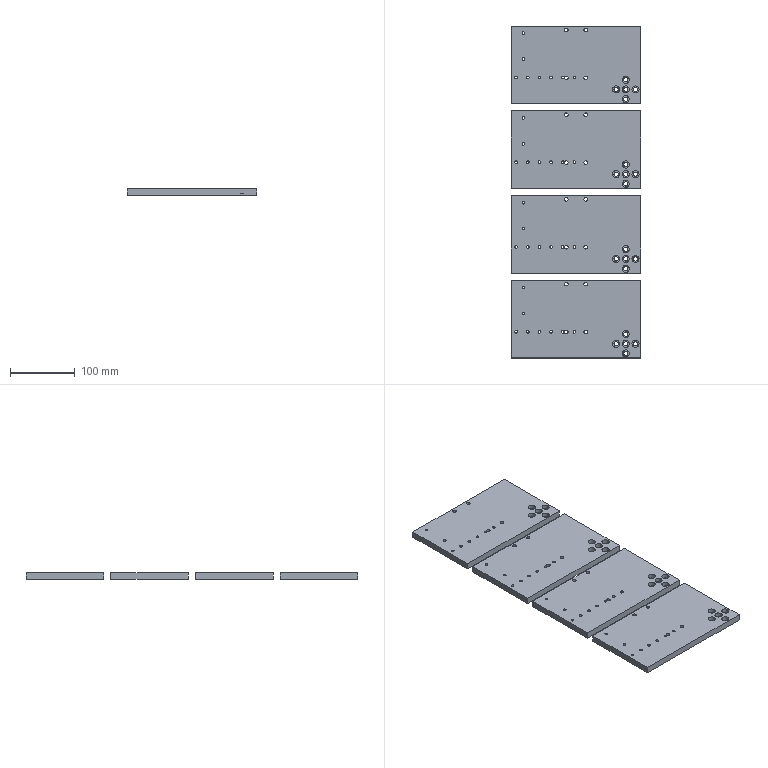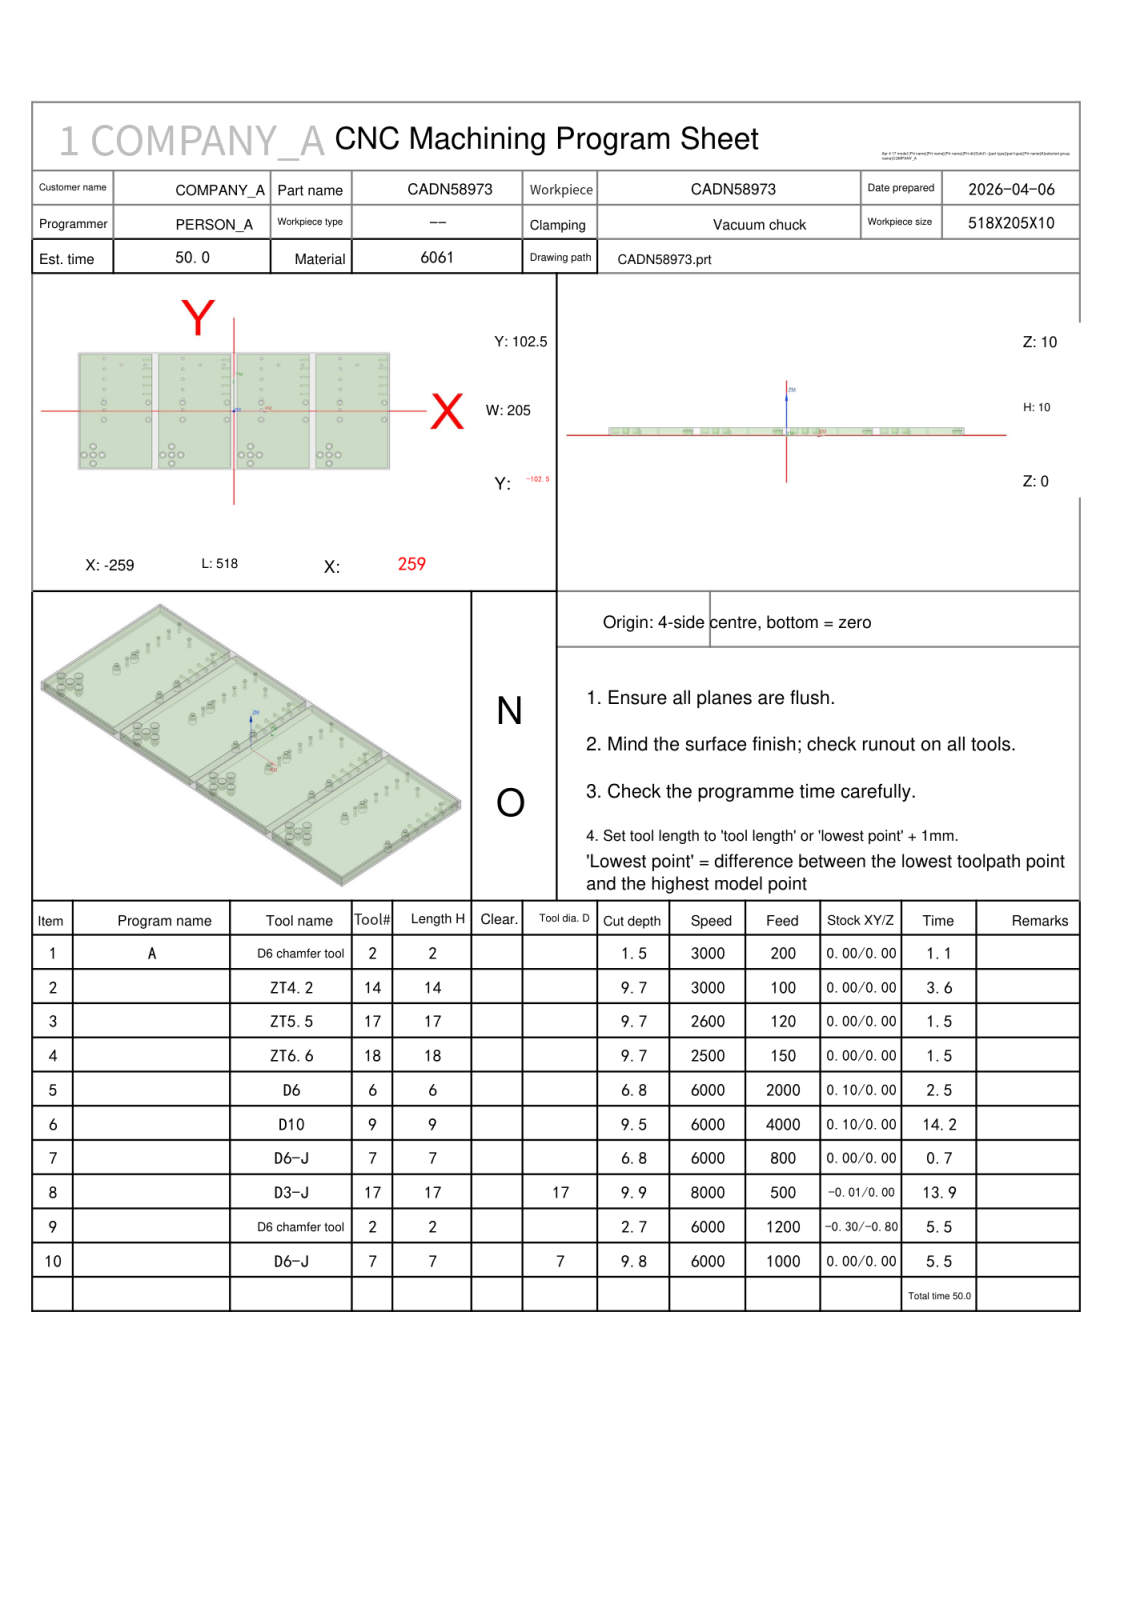NC program | NX | posted by the shop | part box 200 x 513 x 10 mm
Lines 1 to 1767 of 10035, first 1367 of 1765 lines:
%
O0001
(Machine time: 51.42 MIN)
(===Total Tool:7===)
(T2=D6 chamfer tool   D=6.   R=0.   D-  H02 Z=7.33  )
(T14=ZT4.2  D=4.2  DR_a=118 D-  H14 Z=0.3   )
(T17=ZT5.5  D=5.5  DR_a=118 D-  H17 Z=0.15  )
(T18=ZT6.6  D=6.6  DR_a=118 D-  H18 Z=0.3   )
(T6=D6      D=6.   R=0.   D-  H06 Z=3.2   )
(T9=D10     D=10.  R=0.   D-  H09 Z=0.5   )
(T7=D6-J    D=6.   R=0.   D-  H07 Z=0.2   )
G80 G90 G17 G49 G40
G91 G28 Z0
M01
N1 T02 M06
(D6 chamfer tool  D=6. R=0. H=02 ce=0.00 di=0.00)
G00 G90 G54 X-219.5 Y-77. M03 S3000
G43 H02 Z30.
M08
G98 G81 X-219.5 Y-77. Z8.5 R11. F200.
X-234.5
Y-92.
X-249.5 Y-77.
X-234.5 Y-62.
X-216.5 Y-15.
X-216. Y2.515
X-216.5 Y15.
X-216. Y20.515
Y38.515
Y56.515
Y74.515
Y92.515
X-187.5 Y81.264
X-147.5
X-85. Y92.515
X-16.5 Y81.264
X-56.5
X-85. Y74.515
Y56.515
Y38.515
Y20.515
X-85.5 Y15.
X-142.5
Y-15.
X-118.5 Y-77.
X-103.5 Y-92.
X-88.5 Y-77.
X-103.5
Y-62.
X-85.5 Y-15.
X-85. Y2.515
X-11.5 Y15.
Y-15.
X12.5 Y-77.
X27.5
Y-92.
X42.5 Y-77.
X27.5 Y-62.
X45.5 Y-15.
X46. Y2.515
X45.5 Y15.
X46. Y20.515
Y38.515
Y56.515
Y74.515
Y92.515
X74.5 Y81.264
X114.5
X119.5 Y15.
Y-15.
X158.5 Y-62.
Y-77.
X143.5
X158.5 Y-92.
X173.5 Y-77.
X176.5 Y-15.
X177. Y2.515
X176.5 Y15.
X177. Y20.515
Y38.515
Y56.515
Y74.515
Y92.515
X205.5 Y81.264
X245.5
X250.5 Y15.
Y-15.
G80
G00 Z30.
G91 G28 Z0.0
M05
M09
G91 G28 Z0.0
M01
N2 T14 M06
(ZT4.2 D=4.2 DR_a=118 H=14)
G00 G90 G54 X-216. Y2.515 M03 S3000
G43 H14 Z30.
M08
G98 G83 X-216. Y2.515 Z.3 R11. F100. Q1.5
Y20.515
Y38.515
Y56.515
Y74.515
Y92.515
X-187.5 Y81.264
X-147.5
X-85. Y2.515
Y20.515
Y38.515
Y56.515
Y74.515
Y92.515
X-56.5 Y81.264
X-16.5
X46. Y2.515
Y20.515
Y38.515
Y56.515
Y74.515
Y92.515
X74.5 Y81.264
X114.5
X177. Y92.515
X245.5 Y81.264
X205.5
X177. Y74.515
Y56.515
Y38.515
Y20.515
Y2.515
G80
G00 Z30.
G91 G28 Z0.0
M05
M09
G91 G28 Z0.0
M01
N3 T17 M06
(ZT5.5 D=5.5 DR_a=118 H=17)
G00 G90 G54 X250.5 Y15. M03 S2600
G43 H17 Z30.
M08
G98 G83 X250.5 Y15. Z.3 R11. F120. Q1.5
Y-15.
X176.5
Y15.
X119.5
Y-15.
X45.5
Y15.
X-11.5
Y-15.
X-85.5
Y15.
X-142.5
Y-15.
X-216.5
Y15.
G80
G00 Z30.
G91 G28 Z0.0
M05
M09
G91 G28 Z0.0
M01
N4 T18 M06
(ZT6.6 D=6.6 DR_a=118 H=18)
G00 G90 G54 X-234.5 Y-92. M03 S2500
G43 H18 Z30.
M08
G98 G83 X-234.5 Y-92. Z.3 R11. F150. Q3.
X-249.5 Y-77.
X-234.5
Y-62.
X-219.5 Y-77.
X-118.5
X-103.5 Y-62.
Y-77.
Y-92.
X-88.5 Y-77.
X12.5
X27.5 Y-92.
Y-77.
Y-62.
X42.5 Y-77.
X143.5
X158.5 Y-92.
Y-77.
Y-62.
X173.5 Y-77.
G80
G00 Z30.
G91 G28 Z0.0
M05
M09
G91 G28 Z0.0
M01
N5 T06 M06
(D6  D=6. R=0. H=06 ce=0.10 di=0.00)
G00 G90 G54 X42.5 Y-77. M03 S6000
G43 H06 Z30.
M08
Z10.3
G03 X41.3 Y-78.2 I0.0 J-1.2 F2000.
X42.5 Y-79.4 I1.2 J0.0
X42.5 Y-79.4 Z9.8 I0.0 J2.4
X42.5 Y-79.4 Z9.3 I0.0 J2.4
X42.5 Y-79.4 Z8.8 I0.0 J2.4
X42.5 Y-79.4 Z8.3 I0.0 J2.4
X42.5 Y-79.4 Z7.8 I0.0 J2.4
X42.5 Y-79.4 Z7.3 I0.0 J2.4
X42.5 Y-79.4 Z6.8 I0.0 J2.4
X42.5 Y-79.4 Z6.3 I0.0 J2.4
X42.5 Y-79.4 Z5.8 I0.0 J2.4
X42.5 Y-79.4 Z5.3 I0.0 J2.4
X42.5 Y-79.4 Z4.8 I0.0 J2.4
X42.5 Y-79.4 Z4.3 I0.0 J2.4
X42.5 Y-79.4 Z3.8 I0.0 J2.4
X42.5 Y-79.4 Z3.3 I0.0 J2.4
X44.783 Y-77.742 Z3.2 I0.0 J2.4
X44.9 Y-77. I-2.283 J.742
X42.5 Y-74.6 I-2.4 J0.0
X40.1 Y-77. I0.0 J-2.4
X42.5 Y-79.4 I2.4 J0.0
X44.783 Y-77.742 I0.0 J2.4
X44.841 Y-77.371 I-1.141 J.371
X43.641 Y-76.171 I-1.2 J0.0
X42.5 Y-77. I0.0 J-1.2
G00 Z30.
X143.5
Z10.3
G03 X142.3 Y-78.2 I0.0 J-1.2
X143.5 Y-79.4 I1.2 J0.0
X143.5 Y-79.4 Z9.8 I0.0 J2.4
X143.5 Y-79.4 Z9.3 I0.0 J2.4
X143.5 Y-79.4 Z8.8 I0.0 J2.4
X143.5 Y-79.4 Z8.3 I0.0 J2.4
X143.5 Y-79.4 Z7.8 I0.0 J2.4
X143.5 Y-79.4 Z7.3 I0.0 J2.4
X143.5 Y-79.4 Z6.8 I0.0 J2.4
X143.5 Y-79.4 Z6.3 I0.0 J2.4
X143.5 Y-79.4 Z5.8 I0.0 J2.4
X143.5 Y-79.4 Z5.3 I0.0 J2.4
X143.5 Y-79.4 Z4.8 I0.0 J2.4
X143.5 Y-79.4 Z4.3 I0.0 J2.4
X143.5 Y-79.4 Z3.8 I0.0 J2.4
X143.5 Y-79.4 Z3.3 I0.0 J2.4
X145.783 Y-77.742 Z3.2 I0.0 J2.4
X145.9 Y-77. I-2.283 J.742
X143.5 Y-74.6 I-2.4 J0.0
X141.1 Y-77. I0.0 J-2.4
X143.5 Y-79.4 I2.4 J0.0
X145.783 Y-77.742 I0.0 J2.4
X145.841 Y-77.371 I-1.141 J.371
X144.641 Y-76.171 I-1.2 J0.0
X143.5 Y-77. I0.0 J-1.2
G00 Z30.
X158.5 Y-92.
Z10.3
G03 X157.3 Y-93.2 I0.0 J-1.2
X158.5 Y-94.4 I1.2 J0.0
X158.5 Y-94.4 Z9.8 I0.0 J2.4
X158.5 Y-94.4 Z9.3 I0.0 J2.4
X158.5 Y-94.4 Z8.8 I0.0 J2.4
X158.5 Y-94.4 Z8.3 I0.0 J2.4
X158.5 Y-94.4 Z7.8 I0.0 J2.4
X158.5 Y-94.4 Z7.3 I0.0 J2.4
X158.5 Y-94.4 Z6.8 I0.0 J2.4
X158.5 Y-94.4 Z6.3 I0.0 J2.4
X158.5 Y-94.4 Z5.8 I0.0 J2.4
X158.5 Y-94.4 Z5.3 I0.0 J2.4
X158.5 Y-94.4 Z4.8 I0.0 J2.4
X158.5 Y-94.4 Z4.3 I0.0 J2.4
X158.5 Y-94.4 Z3.8 I0.0 J2.4
X158.5 Y-94.4 Z3.3 I0.0 J2.4
X160.783 Y-92.742 Z3.2 I0.0 J2.4
X160.9 Y-92. I-2.283 J.742
X158.5 Y-89.6 I-2.4 J0.0
X156.1 Y-92. I0.0 J-2.4
X158.5 Y-94.4 I2.4 J0.0
X160.783 Y-92.742 I0.0 J2.4
X160.841 Y-92.371 I-1.141 J.371
X159.641 Y-91.171 I-1.2 J0.0
X158.5 Y-92. I0.0 J-1.2
G00 Z30.
Y-77.
Z10.3
G03 X157.3 Y-78.2 I0.0 J-1.2
X158.5 Y-79.4 I1.2 J0.0
X158.5 Y-79.4 Z9.8 I0.0 J2.4
X158.5 Y-79.4 Z9.3 I0.0 J2.4
X158.5 Y-79.4 Z8.8 I0.0 J2.4
X158.5 Y-79.4 Z8.3 I0.0 J2.4
X158.5 Y-79.4 Z7.8 I0.0 J2.4
X158.5 Y-79.4 Z7.3 I0.0 J2.4
X158.5 Y-79.4 Z6.8 I0.0 J2.4
X158.5 Y-79.4 Z6.3 I0.0 J2.4
X158.5 Y-79.4 Z5.8 I0.0 J2.4
X158.5 Y-79.4 Z5.3 I0.0 J2.4
X158.5 Y-79.4 Z4.8 I0.0 J2.4
X158.5 Y-79.4 Z4.3 I0.0 J2.4
X158.5 Y-79.4 Z3.8 I0.0 J2.4
X158.5 Y-79.4 Z3.3 I0.0 J2.4
X160.783 Y-77.742 Z3.2 I0.0 J2.4
X160.9 Y-77. I-2.283 J.742
X158.5 Y-74.6 I-2.4 J0.0
X156.1 Y-77. I0.0 J-2.4
X158.5 Y-79.4 I2.4 J0.0
X160.783 Y-77.742 I0.0 J2.4
X160.841 Y-77.371 I-1.141 J.371
X159.641 Y-76.171 I-1.2 J0.0
X158.5 Y-77. I0.0 J-1.2
G00 Z30.
X173.5
Z10.3
G03 X172.3 Y-78.2 I0.0 J-1.2
X173.5 Y-79.4 I1.2 J0.0
X173.5 Y-79.4 Z9.8 I0.0 J2.4
X173.5 Y-79.4 Z9.3 I0.0 J2.4
X173.5 Y-79.4 Z8.8 I0.0 J2.4
X173.5 Y-79.4 Z8.3 I0.0 J2.4
X173.5 Y-79.4 Z7.8 I0.0 J2.4
X173.5 Y-79.4 Z7.3 I0.0 J2.4
X173.5 Y-79.4 Z6.8 I0.0 J2.4
X173.5 Y-79.4 Z6.3 I0.0 J2.4
X173.5 Y-79.4 Z5.8 I0.0 J2.4
X173.5 Y-79.4 Z5.3 I0.0 J2.4
X173.5 Y-79.4 Z4.8 I0.0 J2.4
X173.5 Y-79.4 Z4.3 I0.0 J2.4
X173.5 Y-79.4 Z3.8 I0.0 J2.4
X173.5 Y-79.4 Z3.3 I0.0 J2.4
X175.783 Y-77.742 Z3.2 I0.0 J2.4
X175.9 Y-77. I-2.283 J.742
X173.5 Y-74.6 I-2.4 J0.0
X171.1 Y-77. I0.0 J-2.4
X173.5 Y-79.4 I2.4 J0.0
X175.783 Y-77.742 I0.0 J2.4
X175.841 Y-77.371 I-1.141 J.371
X174.641 Y-76.171 I-1.2 J0.0
X173.5 Y-77. I0.0 J-1.2
G00 Z30.
X158.5 Y-62.
Z10.3
G03 X157.3 Y-63.2 I0.0 J-1.2
X158.5 Y-64.4 I1.2 J0.0
X158.5 Y-64.4 Z9.8 I0.0 J2.4
X158.5 Y-64.4 Z9.3 I0.0 J2.4
X158.5 Y-64.4 Z8.8 I0.0 J2.4
X158.5 Y-64.4 Z8.3 I0.0 J2.4
X158.5 Y-64.4 Z7.8 I0.0 J2.4
X158.5 Y-64.4 Z7.3 I0.0 J2.4
X158.5 Y-64.4 Z6.8 I0.0 J2.4
X158.5 Y-64.4 Z6.3 I0.0 J2.4
X158.5 Y-64.4 Z5.8 I0.0 J2.4
X158.5 Y-64.4 Z5.3 I0.0 J2.4
X158.5 Y-64.4 Z4.8 I0.0 J2.4
X158.5 Y-64.4 Z4.3 I0.0 J2.4
X158.5 Y-64.4 Z3.8 I0.0 J2.4
X158.5 Y-64.4 Z3.3 I0.0 J2.4
X160.783 Y-62.742 Z3.2 I0.0 J2.4
X160.9 Y-62. I-2.283 J.742
X158.5 Y-59.6 I-2.4 J0.0
X156.1 Y-62. I0.0 J-2.4
X158.5 Y-64.4 I2.4 J0.0
X160.783 Y-62.742 I0.0 J2.4
X160.841 Y-62.371 I-1.141 J.371
X159.641 Y-61.171 I-1.2 J0.0
X158.5 Y-62. I0.0 J-1.2
G00 Z30.
X27.5
Z10.3
G03 X26.3 Y-63.2 I0.0 J-1.2
X27.5 Y-64.4 I1.2 J0.0
X27.5 Y-64.4 Z9.8 I0.0 J2.4
X27.5 Y-64.4 Z9.3 I0.0 J2.4
X27.5 Y-64.4 Z8.8 I0.0 J2.4
X27.5 Y-64.4 Z8.3 I0.0 J2.4
X27.5 Y-64.4 Z7.8 I0.0 J2.4
X27.5 Y-64.4 Z7.3 I0.0 J2.4
X27.5 Y-64.4 Z6.8 I0.0 J2.4
X27.5 Y-64.4 Z6.3 I0.0 J2.4
X27.5 Y-64.4 Z5.8 I0.0 J2.4
X27.5 Y-64.4 Z5.3 I0.0 J2.4
X27.5 Y-64.4 Z4.8 I0.0 J2.4
X27.5 Y-64.4 Z4.3 I0.0 J2.4
X27.5 Y-64.4 Z3.8 I0.0 J2.4
X27.5 Y-64.4 Z3.3 I0.0 J2.4
X29.783 Y-62.742 Z3.2 I0.0 J2.4
X29.9 Y-62. I-2.283 J.742
X27.5 Y-59.6 I-2.4 J0.0
X25.1 Y-62. I0.0 J-2.4
X27.5 Y-64.4 I2.4 J0.0
X29.783 Y-62.742 I0.0 J2.4
X29.841 Y-62.371 I-1.141 J.371
X28.641 Y-61.171 I-1.2 J0.0
X27.5 Y-62. I0.0 J-1.2
G00 Z30.
Y-77.
Z10.3
G03 X26.3 Y-78.2 I0.0 J-1.2
X27.5 Y-79.4 I1.2 J0.0
X27.5 Y-79.4 Z9.8 I0.0 J2.4
X27.5 Y-79.4 Z9.3 I0.0 J2.4
X27.5 Y-79.4 Z8.8 I0.0 J2.4
X27.5 Y-79.4 Z8.3 I0.0 J2.4
X27.5 Y-79.4 Z7.8 I0.0 J2.4
X27.5 Y-79.4 Z7.3 I0.0 J2.4
X27.5 Y-79.4 Z6.8 I0.0 J2.4
X27.5 Y-79.4 Z6.3 I0.0 J2.4
X27.5 Y-79.4 Z5.8 I0.0 J2.4
X27.5 Y-79.4 Z5.3 I0.0 J2.4
X27.5 Y-79.4 Z4.8 I0.0 J2.4
X27.5 Y-79.4 Z4.3 I0.0 J2.4
X27.5 Y-79.4 Z3.8 I0.0 J2.4
X27.5 Y-79.4 Z3.3 I0.0 J2.4
X29.783 Y-77.742 Z3.2 I0.0 J2.4
X29.9 Y-77. I-2.283 J.742
X27.5 Y-74.6 I-2.4 J0.0
X25.1 Y-77. I0.0 J-2.4
X27.5 Y-79.4 I2.4 J0.0
X29.783 Y-77.742 I0.0 J2.4
X29.841 Y-77.371 I-1.141 J.371
X28.641 Y-76.171 I-1.2 J0.0
X27.5 Y-77. I0.0 J-1.2
G00 Z30.
Y-92.
Z10.3
G03 X26.3 Y-93.2 I0.0 J-1.2
X27.5 Y-94.4 I1.2 J0.0
X27.5 Y-94.4 Z9.8 I0.0 J2.4
X27.5 Y-94.4 Z9.3 I0.0 J2.4
X27.5 Y-94.4 Z8.8 I0.0 J2.4
X27.5 Y-94.4 Z8.3 I0.0 J2.4
X27.5 Y-94.4 Z7.8 I0.0 J2.4
X27.5 Y-94.4 Z7.3 I0.0 J2.4
X27.5 Y-94.4 Z6.8 I0.0 J2.4
X27.5 Y-94.4 Z6.3 I0.0 J2.4
X27.5 Y-94.4 Z5.8 I0.0 J2.4
X27.5 Y-94.4 Z5.3 I0.0 J2.4
X27.5 Y-94.4 Z4.8 I0.0 J2.4
X27.5 Y-94.4 Z4.3 I0.0 J2.4
X27.5 Y-94.4 Z3.8 I0.0 J2.4
X27.5 Y-94.4 Z3.3 I0.0 J2.4
X29.783 Y-92.742 Z3.2 I0.0 J2.4
X29.9 Y-92. I-2.283 J.742
X27.5 Y-89.6 I-2.4 J0.0
X25.1 Y-92. I0.0 J-2.4
X27.5 Y-94.4 I2.4 J0.0
X29.783 Y-92.742 I0.0 J2.4
X29.841 Y-92.371 I-1.141 J.371
X28.641 Y-91.171 I-1.2 J0.0
X27.5 Y-92. I0.0 J-1.2
G00 Z30.
X12.5 Y-77.
Z10.3
G03 X11.3 Y-78.2 I0.0 J-1.2
X12.5 Y-79.4 I1.2 J0.0
X12.5 Y-79.4 Z9.8 I0.0 J2.4
X12.5 Y-79.4 Z9.3 I0.0 J2.4
X12.5 Y-79.4 Z8.8 I0.0 J2.4
X12.5 Y-79.4 Z8.3 I0.0 J2.4
X12.5 Y-79.4 Z7.8 I0.0 J2.4
X12.5 Y-79.4 Z7.3 I0.0 J2.4
X12.5 Y-79.4 Z6.8 I0.0 J2.4
X12.5 Y-79.4 Z6.3 I0.0 J2.4
X12.5 Y-79.4 Z5.8 I0.0 J2.4
X12.5 Y-79.4 Z5.3 I0.0 J2.4
X12.5 Y-79.4 Z4.8 I0.0 J2.4
X12.5 Y-79.4 Z4.3 I0.0 J2.4
X12.5 Y-79.4 Z3.8 I0.0 J2.4
X12.5 Y-79.4 Z3.3 I0.0 J2.4
X14.783 Y-77.742 Z3.2 I0.0 J2.4
X14.9 Y-77. I-2.283 J.742
X12.5 Y-74.6 I-2.4 J0.0
X10.1 Y-77. I0.0 J-2.4
X12.5 Y-79.4 I2.4 J0.0
X14.783 Y-77.742 I0.0 J2.4
X14.841 Y-77.371 I-1.141 J.371
X13.641 Y-76.171 I-1.2 J0.0
X12.5 Y-77. I0.0 J-1.2
G00 Z30.
X-88.5
Z10.3
G03 X-89.7 Y-78.2 I0.0 J-1.2
X-88.5 Y-79.4 I1.2 J0.0
X-88.5 Y-79.4 Z9.8 I0.0 J2.4
X-88.5 Y-79.4 Z9.3 I0.0 J2.4
X-88.5 Y-79.4 Z8.8 I0.0 J2.4
X-88.5 Y-79.4 Z8.3 I0.0 J2.4
X-88.5 Y-79.4 Z7.8 I0.0 J2.4
X-88.5 Y-79.4 Z7.3 I0.0 J2.4
X-88.5 Y-79.4 Z6.8 I0.0 J2.4
X-88.5 Y-79.4 Z6.3 I0.0 J2.4
X-88.5 Y-79.4 Z5.8 I0.0 J2.4
X-88.5 Y-79.4 Z5.3 I0.0 J2.4
X-88.5 Y-79.4 Z4.8 I0.0 J2.4
X-88.5 Y-79.4 Z4.3 I0.0 J2.4
X-88.5 Y-79.4 Z3.8 I0.0 J2.4
X-88.5 Y-79.4 Z3.3 I0.0 J2.4
X-86.217 Y-77.742 Z3.2 I0.0 J2.4
X-86.1 Y-77. I-2.283 J.742
X-88.5 Y-74.6 I-2.4 J0.0
X-90.9 Y-77. I0.0 J-2.4
X-88.5 Y-79.4 I2.4 J0.0
X-86.217 Y-77.742 I0.0 J2.4
X-86.159 Y-77.371 I-1.141 J.371
X-87.359 Y-76.171 I-1.2 J0.0
X-88.5 Y-77. I0.0 J-1.2
G00 Z30.
X-103.5 Y-92.
Z10.3
G03 X-104.7 Y-93.2 I0.0 J-1.2
X-103.5 Y-94.4 I1.2 J0.0
X-103.5 Y-94.4 Z9.8 I0.0 J2.4
X-103.5 Y-94.4 Z9.3 I0.0 J2.4
X-103.5 Y-94.4 Z8.8 I0.0 J2.4
X-103.5 Y-94.4 Z8.3 I0.0 J2.4
X-103.5 Y-94.4 Z7.8 I0.0 J2.4
X-103.5 Y-94.4 Z7.3 I0.0 J2.4
X-103.5 Y-94.4 Z6.8 I0.0 J2.4
X-103.5 Y-94.4 Z6.3 I0.0 J2.4
X-103.5 Y-94.4 Z5.8 I0.0 J2.4
X-103.5 Y-94.4 Z5.3 I0.0 J2.4
X-103.5 Y-94.4 Z4.8 I0.0 J2.4
X-103.5 Y-94.4 Z4.3 I0.0 J2.4
X-103.5 Y-94.4 Z3.8 I0.0 J2.4
X-103.5 Y-94.4 Z3.3 I0.0 J2.4
X-101.217 Y-92.742 Z3.2 I0.0 J2.4
X-101.1 Y-92. I-2.283 J.742
X-103.5 Y-89.6 I-2.4 J0.0
X-105.9 Y-92. I0.0 J-2.4
X-103.5 Y-94.4 I2.4 J0.0
X-101.217 Y-92.742 I0.0 J2.4
X-101.159 Y-92.371 I-1.141 J.371
X-102.359 Y-91.171 I-1.2 J0.0
X-103.5 Y-92. I0.0 J-1.2
G00 Z30.
Y-77.
Z10.3
G03 X-104.7 Y-78.2 I0.0 J-1.2
X-103.5 Y-79.4 I1.2 J0.0
X-103.5 Y-79.4 Z9.8 I0.0 J2.4
X-103.5 Y-79.4 Z9.3 I0.0 J2.4
X-103.5 Y-79.4 Z8.8 I0.0 J2.4
X-103.5 Y-79.4 Z8.3 I0.0 J2.4
X-103.5 Y-79.4 Z7.8 I0.0 J2.4
X-103.5 Y-79.4 Z7.3 I0.0 J2.4
X-103.5 Y-79.4 Z6.8 I0.0 J2.4
X-103.5 Y-79.4 Z6.3 I0.0 J2.4
X-103.5 Y-79.4 Z5.8 I0.0 J2.4
X-103.5 Y-79.4 Z5.3 I0.0 J2.4
X-103.5 Y-79.4 Z4.8 I0.0 J2.4
X-103.5 Y-79.4 Z4.3 I0.0 J2.4
X-103.5 Y-79.4 Z3.8 I0.0 J2.4
X-103.5 Y-79.4 Z3.3 I0.0 J2.4
X-101.217 Y-77.742 Z3.2 I0.0 J2.4
X-101.1 Y-77. I-2.283 J.742
X-103.5 Y-74.6 I-2.4 J0.0
X-105.9 Y-77. I0.0 J-2.4
X-103.5 Y-79.4 I2.4 J0.0
X-101.217 Y-77.742 I0.0 J2.4
X-101.159 Y-77.371 I-1.141 J.371
X-102.359 Y-76.171 I-1.2 J0.0
X-103.5 Y-77. I0.0 J-1.2
G00 Z30.
Y-62.
Z10.3
G03 X-104.7 Y-63.2 I0.0 J-1.2
X-103.5 Y-64.4 I1.2 J0.0
X-103.5 Y-64.4 Z9.8 I0.0 J2.4
X-103.5 Y-64.4 Z9.3 I0.0 J2.4
X-103.5 Y-64.4 Z8.8 I0.0 J2.4
X-103.5 Y-64.4 Z8.3 I0.0 J2.4
X-103.5 Y-64.4 Z7.8 I0.0 J2.4
X-103.5 Y-64.4 Z7.3 I0.0 J2.4
X-103.5 Y-64.4 Z6.8 I0.0 J2.4
X-103.5 Y-64.4 Z6.3 I0.0 J2.4
X-103.5 Y-64.4 Z5.8 I0.0 J2.4
X-103.5 Y-64.4 Z5.3 I0.0 J2.4
X-103.5 Y-64.4 Z4.8 I0.0 J2.4
X-103.5 Y-64.4 Z4.3 I0.0 J2.4
X-103.5 Y-64.4 Z3.8 I0.0 J2.4
X-103.5 Y-64.4 Z3.3 I0.0 J2.4
X-101.217 Y-62.742 Z3.2 I0.0 J2.4
X-101.1 Y-62. I-2.283 J.742
X-103.5 Y-59.6 I-2.4 J0.0
X-105.9 Y-62. I0.0 J-2.4
X-103.5 Y-64.4 I2.4 J0.0
X-101.217 Y-62.742 I0.0 J2.4
X-101.159 Y-62.371 I-1.141 J.371
X-102.359 Y-61.171 I-1.2 J0.0
X-103.5 Y-62. I0.0 J-1.2
G00 Z30.
X-118.5 Y-77.
Z10.3
G03 X-119.7 Y-78.2 I0.0 J-1.2
X-118.5 Y-79.4 I1.2 J0.0
X-118.5 Y-79.4 Z9.8 I0.0 J2.4
X-118.5 Y-79.4 Z9.3 I0.0 J2.4
X-118.5 Y-79.4 Z8.8 I0.0 J2.4
X-118.5 Y-79.4 Z8.3 I0.0 J2.4
X-118.5 Y-79.4 Z7.8 I0.0 J2.4
X-118.5 Y-79.4 Z7.3 I0.0 J2.4
X-118.5 Y-79.4 Z6.8 I0.0 J2.4
X-118.5 Y-79.4 Z6.3 I0.0 J2.4
X-118.5 Y-79.4 Z5.8 I0.0 J2.4
X-118.5 Y-79.4 Z5.3 I0.0 J2.4
X-118.5 Y-79.4 Z4.8 I0.0 J2.4
X-118.5 Y-79.4 Z4.3 I0.0 J2.4
X-118.5 Y-79.4 Z3.8 I0.0 J2.4
X-118.5 Y-79.4 Z3.3 I0.0 J2.4
X-116.217 Y-77.742 Z3.2 I0.0 J2.4
X-116.1 Y-77. I-2.283 J.742
X-118.5 Y-74.6 I-2.4 J0.0
X-120.9 Y-77. I0.0 J-2.4
X-118.5 Y-79.4 I2.4 J0.0
X-116.217 Y-77.742 I0.0 J2.4
X-116.159 Y-77.371 I-1.141 J.371
X-117.359 Y-76.171 I-1.2 J0.0
X-118.5 Y-77. I0.0 J-1.2
G00 Z30.
X-219.5
Z10.3
G03 X-220.7 Y-78.2 I0.0 J-1.2
X-219.5 Y-79.4 I1.2 J0.0
X-219.5 Y-79.4 Z9.8 I0.0 J2.4
X-219.5 Y-79.4 Z9.3 I0.0 J2.4
X-219.5 Y-79.4 Z8.8 I0.0 J2.4
X-219.5 Y-79.4 Z8.3 I0.0 J2.4
X-219.5 Y-79.4 Z7.8 I0.0 J2.4
X-219.5 Y-79.4 Z7.3 I0.0 J2.4
X-219.5 Y-79.4 Z6.8 I0.0 J2.4
X-219.5 Y-79.4 Z6.3 I0.0 J2.4
X-219.5 Y-79.4 Z5.8 I0.0 J2.4
X-219.5 Y-79.4 Z5.3 I0.0 J2.4
X-219.5 Y-79.4 Z4.8 I0.0 J2.4
X-219.5 Y-79.4 Z4.3 I0.0 J2.4
X-219.5 Y-79.4 Z3.8 I0.0 J2.4
X-219.5 Y-79.4 Z3.3 I0.0 J2.4
X-217.217 Y-77.742 Z3.2 I0.0 J2.4
X-217.1 Y-77. I-2.283 J.742
X-219.5 Y-74.6 I-2.4 J0.0
X-221.9 Y-77. I0.0 J-2.4
X-219.5 Y-79.4 I2.4 J0.0
X-217.217 Y-77.742 I0.0 J2.4
X-217.159 Y-77.371 I-1.141 J.371
X-218.359 Y-76.171 I-1.2 J0.0
X-219.5 Y-77. I0.0 J-1.2
G00 Z30.
X-234.5 Y-92.
Z10.3
G03 X-235.7 Y-93.2 I0.0 J-1.2
X-234.5 Y-94.4 I1.2 J0.0
X-234.5 Y-94.4 Z9.8 I0.0 J2.4
X-234.5 Y-94.4 Z9.3 I0.0 J2.4
X-234.5 Y-94.4 Z8.8 I0.0 J2.4
X-234.5 Y-94.4 Z8.3 I0.0 J2.4
X-234.5 Y-94.4 Z7.8 I0.0 J2.4
X-234.5 Y-94.4 Z7.3 I0.0 J2.4
X-234.5 Y-94.4 Z6.8 I0.0 J2.4
X-234.5 Y-94.4 Z6.3 I0.0 J2.4
X-234.5 Y-94.4 Z5.8 I0.0 J2.4
X-234.5 Y-94.4 Z5.3 I0.0 J2.4
X-234.5 Y-94.4 Z4.8 I0.0 J2.4
X-234.5 Y-94.4 Z4.3 I0.0 J2.4
X-234.5 Y-94.4 Z3.8 I0.0 J2.4
X-234.5 Y-94.4 Z3.3 I0.0 J2.4
X-232.217 Y-92.742 Z3.2 I0.0 J2.4
X-232.1 Y-92. I-2.283 J.742
X-234.5 Y-89.6 I-2.4 J0.0
X-236.9 Y-92. I0.0 J-2.4
X-234.5 Y-94.4 I2.4 J0.0
X-232.217 Y-92.742 I0.0 J2.4
X-232.159 Y-92.371 I-1.141 J.371
X-233.359 Y-91.171 I-1.2 J0.0
X-234.5 Y-92. I0.0 J-1.2
G00 Z30.
X-249.5 Y-77.
Z10.3
G03 X-250.7 Y-78.2 I0.0 J-1.2
X-249.5 Y-79.4 I1.2 J0.0
X-249.5 Y-79.4 Z9.8 I0.0 J2.4
X-249.5 Y-79.4 Z9.3 I0.0 J2.4
X-249.5 Y-79.4 Z8.8 I0.0 J2.4
X-249.5 Y-79.4 Z8.3 I0.0 J2.4
X-249.5 Y-79.4 Z7.8 I0.0 J2.4
X-249.5 Y-79.4 Z7.3 I0.0 J2.4
X-249.5 Y-79.4 Z6.8 I0.0 J2.4
X-249.5 Y-79.4 Z6.3 I0.0 J2.4
X-249.5 Y-79.4 Z5.8 I0.0 J2.4
X-249.5 Y-79.4 Z5.3 I0.0 J2.4
X-249.5 Y-79.4 Z4.8 I0.0 J2.4
X-249.5 Y-79.4 Z4.3 I0.0 J2.4
X-249.5 Y-79.4 Z3.8 I0.0 J2.4
X-249.5 Y-79.4 Z3.3 I0.0 J2.4
X-247.217 Y-77.742 Z3.2 I0.0 J2.4
X-247.1 Y-77. I-2.283 J.742
X-249.5 Y-74.6 I-2.4 J0.0
X-251.9 Y-77. I0.0 J-2.4
X-249.5 Y-79.4 I2.4 J0.0
X-247.217 Y-77.742 I0.0 J2.4
X-247.159 Y-77.371 I-1.141 J.371
X-248.359 Y-76.171 I-1.2 J0.0
X-249.5 Y-77. I0.0 J-1.2
G00 Z30.
X-234.5
Z10.3
G03 X-235.7 Y-78.2 I0.0 J-1.2
X-234.5 Y-79.4 I1.2 J0.0
X-234.5 Y-79.4 Z9.8 I0.0 J2.4
X-234.5 Y-79.4 Z9.3 I0.0 J2.4
X-234.5 Y-79.4 Z8.8 I0.0 J2.4
X-234.5 Y-79.4 Z8.3 I0.0 J2.4
X-234.5 Y-79.4 Z7.8 I0.0 J2.4
X-234.5 Y-79.4 Z7.3 I0.0 J2.4
X-234.5 Y-79.4 Z6.8 I0.0 J2.4
X-234.5 Y-79.4 Z6.3 I0.0 J2.4
X-234.5 Y-79.4 Z5.8 I0.0 J2.4
X-234.5 Y-79.4 Z5.3 I0.0 J2.4
X-234.5 Y-79.4 Z4.8 I0.0 J2.4
X-234.5 Y-79.4 Z4.3 I0.0 J2.4
X-234.5 Y-79.4 Z3.8 I0.0 J2.4
X-234.5 Y-79.4 Z3.3 I0.0 J2.4
X-232.217 Y-77.742 Z3.2 I0.0 J2.4
X-232.1 Y-77. I-2.283 J.742
X-234.5 Y-74.6 I-2.4 J0.0
X-236.9 Y-77. I0.0 J-2.4
X-234.5 Y-79.4 I2.4 J0.0
X-232.217 Y-77.742 I0.0 J2.4
X-232.159 Y-77.371 I-1.141 J.371
X-233.359 Y-76.171 I-1.2 J0.0
X-234.5 Y-77. I0.0 J-1.2
G00 Z30.
Y-62.
Z10.3
G03 X-235.7 Y-63.2 I0.0 J-1.2
X-234.5 Y-64.4 I1.2 J0.0
X-234.5 Y-64.4 Z9.8 I0.0 J2.4
X-234.5 Y-64.4 Z9.3 I0.0 J2.4
X-234.5 Y-64.4 Z8.8 I0.0 J2.4
X-234.5 Y-64.4 Z8.3 I0.0 J2.4
X-234.5 Y-64.4 Z7.8 I0.0 J2.4
X-234.5 Y-64.4 Z7.3 I0.0 J2.4
X-234.5 Y-64.4 Z6.8 I0.0 J2.4
X-234.5 Y-64.4 Z6.3 I0.0 J2.4
X-234.5 Y-64.4 Z5.8 I0.0 J2.4
X-234.5 Y-64.4 Z5.3 I0.0 J2.4
X-234.5 Y-64.4 Z4.8 I0.0 J2.4
X-234.5 Y-64.4 Z4.3 I0.0 J2.4
X-234.5 Y-64.4 Z3.8 I0.0 J2.4
X-234.5 Y-64.4 Z3.3 I0.0 J2.4
X-232.217 Y-62.742 Z3.2 I0.0 J2.4
X-232.1 Y-62. I-2.283 J.742
X-234.5 Y-59.6 I-2.4 J0.0
X-236.9 Y-62. I0.0 J-2.4
X-234.5 Y-64.4 I2.4 J0.0
X-232.217 Y-62.742 I0.0 J2.4
X-232.159 Y-62.371 I-1.141 J.371
X-233.359 Y-61.171 I-1.2 J0.0
X-234.5 Y-62. I0.0 J-1.2
G00 Z30.
G91 G28 Z0.0
M05
M09
G91 G28 Z0.0
M01
N6 T09 M06
(D10  D=10. R=0. H=09 ce=0.10 di=0.00)
G00 G90 G54 X.4 Y0.0 M03 S6000
G43 H09 Z30.
M08
Z10.5
G01 Y100. Z10.426 F4000.
G02 X5.5 Y105.1 Z10.42 I5.1 J0.0
G01 X125.5 Z10.33
G02 X130.6 Y100. Z10.324 I0.0 J-5.1
G01 Y-100. Z10.176
G02 X125.5 Y-105.1 Z10.17 I-5.1 J0.0
G01 X5.5 Z10.08
G02 X.4 Y-100. Z10.074 I0.0 J5.1
G01 Y100. Z9.926
G02 X5.5 Y105.1 Z9.92 I5.1 J0.0
G01 X125.5 Z9.83
G02 X130.6 Y100. Z9.824 I0.0 J-5.1
G01 Y-100. Z9.676
G02 X125.5 Y-105.1 Z9.67 I-5.1 J0.0
G01 X5.5 Z9.58
G02 X.4 Y-100. Z9.574 I0.0 J5.1
G01 Y100. Z9.426
G02 X5.5 Y105.1 Z9.42 I5.1 J0.0
G01 X125.5 Z9.33
G02 X130.6 Y100. Z9.324 I0.0 J-5.1
G01 Y-100. Z9.176
G02 X125.5 Y-105.1 Z9.17 I-5.1 J0.0
G01 X5.5 Z9.08
G02 X.4 Y-100. Z9.074 I0.0 J5.1
G01 Y100. Z8.926
G02 X5.5 Y105.1 Z8.92 I5.1 J0.0
G01 X125.5 Z8.83
G02 X130.6 Y100. Z8.824 I0.0 J-5.1
G01 Y-100. Z8.676
G02 X125.5 Y-105.1 Z8.67 I-5.1 J0.0
G01 X5.5 Z8.58
G02 X.4 Y-100. Z8.574 I0.0 J5.1
G01 Y100. Z8.426
G02 X5.5 Y105.1 Z8.42 I5.1 J0.0
G01 X125.5 Z8.33
G02 X130.6 Y100. Z8.324 I0.0 J-5.1
G01 Y-100. Z8.176
G02 X125.5 Y-105.1 Z8.17 I-5.1 J0.0
G01 X5.5 Z8.08
G02 X.4 Y-100. Z8.074 I0.0 J5.1
G01 Y100. Z7.926
G02 X5.5 Y105.1 Z7.92 I5.1 J0.0
G01 X125.5 Z7.83
G02 X130.6 Y100. Z7.824 I0.0 J-5.1
G01 Y-100. Z7.676
G02 X125.5 Y-105.1 Z7.67 I-5.1 J0.0
G01 X5.5 Z7.58
G02 X.4 Y-100. Z7.574 I0.0 J5.1
G01 Y100. Z7.426
G02 X5.5 Y105.1 Z7.42 I5.1 J0.0
G01 X125.5 Z7.33
G02 X130.6 Y100. Z7.324 I0.0 J-5.1
G01 Y-100. Z7.176
G02 X125.5 Y-105.1 Z7.17 I-5.1 J0.0
G01 X5.5 Z7.08
G02 X.4 Y-100. Z7.074 I0.0 J5.1
G01 Y100. Z6.926
G02 X5.5 Y105.1 Z6.92 I5.1 J0.0
G01 X125.5 Z6.83
G02 X130.6 Y100. Z6.824 I0.0 J-5.1
G01 Y-100. Z6.676
G02 X125.5 Y-105.1 Z6.67 I-5.1 J0.0
G01 X5.5 Z6.58
G02 X.4 Y-100. Z6.574 I0.0 J5.1
G01 Y100. Z6.426
G02 X5.5 Y105.1 Z6.42 I5.1 J0.0
G01 X125.5 Z6.33
G02 X130.6 Y100. Z6.324 I0.0 J-5.1
G01 Y-100. Z6.176
G02 X125.5 Y-105.1 Z6.17 I-5.1 J0.0
G01 X5.5 Z6.08
G02 X.4 Y-100. Z6.074 I0.0 J5.1
G01 Y100. Z5.926
G02 X5.5 Y105.1 Z5.92 I5.1 J0.0
G01 X125.5 Z5.83
G02 X130.6 Y100. Z5.824 I0.0 J-5.1
G01 Y-100. Z5.676
G02 X125.5 Y-105.1 Z5.67 I-5.1 J0.0
G01 X5.5 Z5.58
G02 X.4 Y-100. Z5.574 I0.0 J5.1
G01 Y100. Z5.426
G02 X5.5 Y105.1 Z5.42 I5.1 J0.0
G01 X125.5 Z5.33
G02 X130.6 Y100. Z5.324 I0.0 J-5.1
G01 Y-100. Z5.176
G02 X125.5 Y-105.1 Z5.17 I-5.1 J0.0
G01 X5.5 Z5.08
G02 X.4 Y-100. Z5.074 I0.0 J5.1
G01 Y100. Z4.926
G02 X5.5 Y105.1 Z4.92 I5.1 J0.0
G01 X125.5 Z4.83
G02 X130.6 Y100. Z4.824 I0.0 J-5.1
G01 Y-100. Z4.676
G02 X125.5 Y-105.1 Z4.67 I-5.1 J0.0
G01 X5.5 Z4.58
G02 X.4 Y-100. Z4.574 I0.0 J5.1
G01 Y100. Z4.426
G02 X5.5 Y105.1 Z4.42 I5.1 J0.0
G01 X125.5 Z4.33
G02 X130.6 Y100. Z4.324 I0.0 J-5.1
G01 Y-100. Z4.176
G02 X125.5 Y-105.1 Z4.17 I-5.1 J0.0
G01 X5.5 Z4.08
G02 X.4 Y-100. Z4.074 I0.0 J5.1
G01 Y100. Z3.926
G02 X5.5 Y105.1 Z3.92 I5.1 J0.0
G01 X125.5 Z3.83
G02 X130.6 Y100. Z3.824 I0.0 J-5.1
G01 Y-100. Z3.676
G02 X125.5 Y-105.1 Z3.67 I-5.1 J0.0
G01 X5.5 Z3.58
G02 X.4 Y-100. Z3.574 I0.0 J5.1
G01 Y100. Z3.426
G02 X5.5 Y105.1 Z3.42 I5.1 J0.0
G01 X125.5 Z3.33
G02 X130.6 Y100. Z3.324 I0.0 J-5.1
G01 Y-100. Z3.176
G02 X125.5 Y-105.1 Z3.17 I-5.1 J0.0
G01 X5.5 Z3.08
G02 X.4 Y-100. Z3.074 I0.0 J5.1
G01 Y100. Z2.926
G02 X5.5 Y105.1 Z2.92 I5.1 J0.0
G01 X125.5 Z2.83
G02 X130.6 Y100. Z2.824 I0.0 J-5.1
G01 Y-100. Z2.676
G02 X125.5 Y-105.1 Z2.67 I-5.1 J0.0
G01 X5.5 Z2.58
G02 X.4 Y-100. Z2.574 I0.0 J5.1
G01 Y100. Z2.426
G02 X5.5 Y105.1 Z2.42 I5.1 J0.0
G01 X125.5 Z2.33
G02 X130.6 Y100. Z2.324 I0.0 J-5.1
G01 Y-100. Z2.176
G02 X125.5 Y-105.1 Z2.17 I-5.1 J0.0
G01 X5.5 Z2.08
G02 X.4 Y-100. Z2.074 I0.0 J5.1
G01 Y100. Z1.926
G02 X5.5 Y105.1 Z1.92 I5.1 J0.0
G01 X125.5 Z1.83
G02 X130.6 Y100. Z1.824 I0.0 J-5.1
G01 Y-100. Z1.676
G02 X125.5 Y-105.1 Z1.67 I-5.1 J0.0
G01 X5.5 Z1.58
G02 X.4 Y-100. Z1.574 I0.0 J5.1
G01 Y100. Z1.426
G02 X5.5 Y105.1 Z1.42 I5.1 J0.0
G01 X125.5 Z1.33
G02 X130.6 Y100. Z1.324 I0.0 J-5.1
G01 Y-100. Z1.176
G02 X125.5 Y-105.1 Z1.17 I-5.1 J0.0
G01 X5.5 Z1.08
G02 X.4 Y-100. Z1.074 I0.0 J5.1
G01 Y100. Z.926
G02 X5.5 Y105.1 Z.92 I5.1 J0.0
G01 X125.5 Z.83
G02 X130.6 Y100. Z.824 I0.0 J-5.1
G01 Y-100. Z.676
G02 X125.5 Y-105.1 Z.67 I-5.1 J0.0
G01 X5.5 Z.58
G02 X.4 Y-100. Z.574 I0.0 J5.1
G01 Y0.0 Z.5
Y100.
G02 X5.5 Y105.1 I5.1 J0.0
G01 X125.5
G02 X130.6 Y100. I0.0 J-5.1
G01 Y-100.
G02 X125.5 Y-105.1 I-5.1 J0.0
G01 X5.5
G02 X.4 Y-100. I0.0 J5.1
G01 Y0.0
Y.5
Z1.5
G00 Z30.
X-.4 Y0.0
Z10.5
G01 Y-100. Z10.426
G02 X-5.5 Y-105.1 Z10.42 I-5.1 J0.0
G01 X-125.5 Z10.33
G02 X-130.6 Y-100. Z10.324 I0.0 J5.1
G01 Y100. Z10.176
G02 X-125.5 Y105.1 Z10.17 I5.1 J0.0
G01 X-5.5 Z10.08
G02 X-.4 Y100. Z10.074 I0.0 J-5.1
G01 Y-100. Z9.926
G02 X-5.5 Y-105.1 Z9.92 I-5.1 J0.0
G01 X-125.5 Z9.83
G02 X-130.6 Y-100. Z9.824 I0.0 J5.1
G01 Y100. Z9.676
G02 X-125.5 Y105.1 Z9.67 I5.1 J0.0
G01 X-5.5 Z9.58
G02 X-.4 Y100. Z9.574 I0.0 J-5.1
G01 Y-100. Z9.426
G02 X-5.5 Y-105.1 Z9.42 I-5.1 J0.0
G01 X-125.5 Z9.33
G02 X-130.6 Y-100. Z9.324 I0.0 J5.1
G01 Y100. Z9.176
G02 X-125.5 Y105.1 Z9.17 I5.1 J0.0
G01 X-5.5 Z9.08
G02 X-.4 Y100. Z9.074 I0.0 J-5.1
G01 Y-100. Z8.926
G02 X-5.5 Y-105.1 Z8.92 I-5.1 J0.0
G01 X-125.5 Z8.83
G02 X-130.6 Y-100. Z8.824 I0.0 J5.1
G01 Y100. Z8.676
G02 X-125.5 Y105.1 Z8.67 I5.1 J0.0
G01 X-5.5 Z8.58
G02 X-.4 Y100. Z8.574 I0.0 J-5.1
G01 Y-100. Z8.426
G02 X-5.5 Y-105.1 Z8.42 I-5.1 J0.0
G01 X-125.5 Z8.33
G02 X-130.6 Y-100. Z8.324 I0.0 J5.1
G01 Y100. Z8.176
G02 X-125.5 Y105.1 Z8.17 I5.1 J0.0
G01 X-5.5 Z8.08
G02 X-.4 Y100. Z8.074 I0.0 J-5.1
G01 Y-100. Z7.926
G02 X-5.5 Y-105.1 Z7.92 I-5.1 J0.0
G01 X-125.5 Z7.83
G02 X-130.6 Y-100. Z7.824 I0.0 J5.1
G01 Y100. Z7.676
G02 X-125.5 Y105.1 Z7.67 I5.1 J0.0
G01 X-5.5 Z7.58
G02 X-.4 Y100. Z7.574 I0.0 J-5.1
G01 Y-100. Z7.426
G02 X-5.5 Y-105.1 Z7.42 I-5.1 J0.0
G01 X-125.5 Z7.33
G02 X-130.6 Y-100. Z7.324 I0.0 J5.1
G01 Y100. Z7.176
G02 X-125.5 Y105.1 Z7.17 I5.1 J0.0
G01 X-5.5 Z7.08
G02 X-.4 Y100. Z7.074 I0.0 J-5.1
G01 Y-100. Z6.926
G02 X-5.5 Y-105.1 Z6.92 I-5.1 J0.0
G01 X-125.5 Z6.83
G02 X-130.6 Y-100. Z6.824 I0.0 J5.1
G01 Y100. Z6.676
G02 X-125.5 Y105.1 Z6.67 I5.1 J0.0
G01 X-5.5 Z6.58
G02 X-.4 Y100. Z6.574 I0.0 J-5.1
G01 Y-100. Z6.426
G02 X-5.5 Y-105.1 Z6.42 I-5.1 J0.0
G01 X-125.5 Z6.33
G02 X-130.6 Y-100. Z6.324 I0.0 J5.1
G01 Y100. Z6.176
G02 X-125.5 Y105.1 Z6.17 I5.1 J0.0
G01 X-5.5 Z6.08
G02 X-.4 Y100. Z6.074 I0.0 J-5.1
G01 Y-100. Z5.926
G02 X-5.5 Y-105.1 Z5.92 I-5.1 J0.0
G01 X-125.5 Z5.83
G02 X-130.6 Y-100. Z5.824 I0.0 J5.1
G01 Y100. Z5.676
G02 X-125.5 Y105.1 Z5.67 I5.1 J0.0
G01 X-5.5 Z5.58
G02 X-.4 Y100. Z5.574 I0.0 J-5.1
G01 Y-100. Z5.426
G02 X-5.5 Y-105.1 Z5.42 I-5.1 J0.0
G01 X-125.5 Z5.33
G02 X-130.6 Y-100. Z5.324 I0.0 J5.1
G01 Y100. Z5.176
G02 X-125.5 Y105.1 Z5.17 I5.1 J0.0
G01 X-5.5 Z5.08
G02 X-.4 Y100. Z5.074 I0.0 J-5.1
G01 Y-100. Z4.926
G02 X-5.5 Y-105.1 Z4.92 I-5.1 J0.0
G01 X-125.5 Z4.83
G02 X-130.6 Y-100. Z4.824 I0.0 J5.1
G01 Y100. Z4.676
G02 X-125.5 Y105.1 Z4.67 I5.1 J0.0
G01 X-5.5 Z4.58
G02 X-.4 Y100. Z4.574 I0.0 J-5.1
G01 Y-100. Z4.426
G02 X-5.5 Y-105.1 Z4.42 I-5.1 J0.0
G01 X-125.5 Z4.33
G02 X-130.6 Y-100. Z4.324 I0.0 J5.1
G01 Y100. Z4.176
G02 X-125.5 Y105.1 Z4.17 I5.1 J0.0
G01 X-5.5 Z4.08
G02 X-.4 Y100. Z4.074 I0.0 J-5.1
G01 Y-100. Z3.926
G02 X-5.5 Y-105.1 Z3.92 I-5.1 J0.0
G01 X-125.5 Z3.83
G02 X-130.6 Y-100. Z3.824 I0.0 J5.1
G01 Y100. Z3.676
G02 X-125.5 Y105.1 Z3.67 I5.1 J0.0
G01 X-5.5 Z3.58
G02 X-.4 Y100. Z3.574 I0.0 J-5.1
G01 Y-100. Z3.426
G02 X-5.5 Y-105.1 Z3.42 I-5.1 J0.0
G01 X-125.5 Z3.33
G02 X-130.6 Y-100. Z3.324 I0.0 J5.1
G01 Y100. Z3.176
G02 X-125.5 Y105.1 Z3.17 I5.1 J0.0
G01 X-5.5 Z3.08
G02 X-.4 Y100. Z3.074 I0.0 J-5.1
G01 Y-100. Z2.926
G02 X-5.5 Y-105.1 Z2.92 I-5.1 J0.0
G01 X-125.5 Z2.83
G02 X-130.6 Y-100. Z2.824 I0.0 J5.1
G01 Y100. Z2.676
G02 X-125.5 Y105.1 Z2.67 I5.1 J0.0
G01 X-5.5 Z2.58
G02 X-.4 Y100. Z2.574 I0.0 J-5.1
G01 Y-100. Z2.426
G02 X-5.5 Y-105.1 Z2.42 I-5.1 J0.0
G01 X-125.5 Z2.33
G02 X-130.6 Y-100. Z2.324 I0.0 J5.1
G01 Y100. Z2.176
G02 X-125.5 Y105.1 Z2.17 I5.1 J0.0
G01 X-5.5 Z2.08
G02 X-.4 Y100. Z2.074 I0.0 J-5.1
G01 Y-100. Z1.926
G02 X-5.5 Y-105.1 Z1.92 I-5.1 J0.0
G01 X-125.5 Z1.83
G02 X-130.6 Y-100. Z1.824 I0.0 J5.1
G01 Y100. Z1.676
G02 X-125.5 Y105.1 Z1.67 I5.1 J0.0
G01 X-5.5 Z1.58
G02 X-.4 Y100. Z1.574 I0.0 J-5.1
G01 Y-100. Z1.426
G02 X-5.5 Y-105.1 Z1.42 I-5.1 J0.0
G01 X-125.5 Z1.33
G02 X-130.6 Y-100. Z1.324 I0.0 J5.1
G01 Y100. Z1.176
G02 X-125.5 Y105.1 Z1.17 I5.1 J0.0
G01 X-5.5 Z1.08
G02 X-.4 Y100. Z1.074 I0.0 J-5.1
G01 Y-100. Z.926
G02 X-5.5 Y-105.1 Z.92 I-5.1 J0.0
G01 X-125.5 Z.83
G02 X-130.6 Y-100. Z.824 I0.0 J5.1
G01 Y100. Z.676
G02 X-125.5 Y105.1 Z.67 I5.1 J0.0
G01 X-5.5 Z.58
G02 X-.4 Y100. Z.574 I0.0 J-5.1
G01 Y0.0 Z.5
Y-100.
G02 X-5.5 Y-105.1 I-5.1 J0.0
G01 X-125.5
G02 X-130.6 Y-100. I0.0 J5.1
G01 Y100.
G02 X-125.5 Y105.1 I5.1 J0.0
G01 X-5.5
G02 X-.4 Y100. I0.0 J-5.1
G01 Y0.0
Y-.5
Z1.5
G00 Z30.
X-261.6 Y0.0
Z10.5
G01 Y100. Z10.426
G02 X-256.5 Y105.1 Z10.42 I5.1 J0.0
G01 X-136.5 Z10.33
G02 X-131.4 Y100. Z10.324 I0.0 J-5.1
G01 Y-100. Z10.176
G02 X-136.5 Y-105.1 Z10.17 I-5.1 J0.0
G01 X-256.5 Z10.08
G02 X-261.6 Y-100. Z10.074 I0.0 J5.1
G01 Y100. Z9.926
G02 X-256.5 Y105.1 Z9.92 I5.1 J0.0
G01 X-136.5 Z9.83
G02 X-131.4 Y100. Z9.824 I0.0 J-5.1
G01 Y-100. Z9.676
G02 X-136.5 Y-105.1 Z9.67 I-5.1 J0.0
G01 X-256.5 Z9.58
G02 X-261.6 Y-100. Z9.574 I0.0 J5.1
G01 Y100. Z9.426
G02 X-256.5 Y105.1 Z9.42 I5.1 J0.0
G01 X-136.5 Z9.33
G02 X-131.4 Y100. Z9.324 I0.0 J-5.1
G01 Y-100. Z9.176
G02 X-136.5 Y-105.1 Z9.17 I-5.1 J0.0
G01 X-256.5 Z9.08
G02 X-261.6 Y-100. Z9.074 I0.0 J5.1
G01 Y100. Z8.926
G02 X-256.5 Y105.1 Z8.92 I5.1 J0.0
G01 X-136.5 Z8.83
G02 X-131.4 Y100. Z8.824 I0.0 J-5.1
G01 Y-100. Z8.676
G02 X-136.5 Y-105.1 Z8.67 I-5.1 J0.0
G01 X-256.5 Z8.58
G02 X-261.6 Y-100. Z8.574 I0.0 J5.1
G01 Y100. Z8.426
G02 X-256.5 Y105.1 Z8.42 I5.1 J0.0
G01 X-136.5 Z8.33
G02 X-131.4 Y100. Z8.324 I0.0 J-5.1
G01 Y-100. Z8.176
G02 X-136.5 Y-105.1 Z8.17 I-5.1 J0.0
G01 X-256.5 Z8.08
G02 X-261.6 Y-100. Z8.074 I0.0 J5.1
G01 Y100. Z7.926
G02 X-256.5 Y105.1 Z7.92 I5.1 J0.0
G01 X-136.5 Z7.83
G02 X-131.4 Y100. Z7.824 I0.0 J-5.1
G01 Y-100. Z7.676
G02 X-136.5 Y-105.1 Z7.67 I-5.1 J0.0
G01 X-256.5 Z7.58
G02 X-261.6 Y-100. Z7.574 I0.0 J5.1
G01 Y100. Z7.426
G02 X-256.5 Y105.1 Z7.42 I5.1 J0.0
G01 X-136.5 Z7.33
G02 X-131.4 Y100. Z7.324 I0.0 J-5.1
G01 Y-100. Z7.176
G02 X-136.5 Y-105.1 Z7.17 I-5.1 J0.0
G01 X-256.5 Z7.08
G02 X-261.6 Y-100. Z7.074 I0.0 J5.1
G01 Y100. Z6.926
G02 X-256.5 Y105.1 Z6.92 I5.1 J0.0
G01 X-136.5 Z6.83
G02 X-131.4 Y100. Z6.824 I0.0 J-5.1
G01 Y-100. Z6.676
G02 X-136.5 Y-105.1 Z6.67 I-5.1 J0.0
G01 X-256.5 Z6.58
G02 X-261.6 Y-100. Z6.574 I0.0 J5.1
G01 Y100. Z6.426
G02 X-256.5 Y105.1 Z6.42 I5.1 J0.0
G01 X-136.5 Z6.33
G02 X-131.4 Y100. Z6.324 I0.0 J-5.1
G01 Y-100. Z6.176
G02 X-136.5 Y-105.1 Z6.17 I-5.1 J0.0
G01 X-256.5 Z6.08
G02 X-261.6 Y-100. Z6.074 I0.0 J5.1
G01 Y100. Z5.926
G02 X-256.5 Y105.1 Z5.92 I5.1 J0.0
G01 X-136.5 Z5.83
G02 X-131.4 Y100. Z5.824 I0.0 J-5.1
G01 Y-100. Z5.676
G02 X-136.5 Y-105.1 Z5.67 I-5.1 J0.0
G01 X-256.5 Z5.58
G02 X-261.6 Y-100. Z5.574 I0.0 J5.1
G01 Y100. Z5.426
G02 X-256.5 Y105.1 Z5.42 I5.1 J0.0
G01 X-136.5 Z5.33
G02 X-131.4 Y100. Z5.324 I0.0 J-5.1
G01 Y-100. Z5.176
G02 X-136.5 Y-105.1 Z5.17 I-5.1 J0.0
G01 X-256.5 Z5.08
G02 X-261.6 Y-100. Z5.074 I0.0 J5.1
G01 Y100. Z4.926
G02 X-256.5 Y105.1 Z4.92 I5.1 J0.0
G01 X-136.5 Z4.83
G02 X-131.4 Y100. Z4.824 I0.0 J-5.1
G01 Y-100. Z4.676
G02 X-136.5 Y-105.1 Z4.67 I-5.1 J0.0
G01 X-256.5 Z4.58
G02 X-261.6 Y-100. Z4.574 I0.0 J5.1
G01 Y100. Z4.426
G02 X-256.5 Y105.1 Z4.42 I5.1 J0.0
G01 X-136.5 Z4.33
G02 X-131.4 Y100. Z4.324 I0.0 J-5.1
G01 Y-100. Z4.176
G02 X-136.5 Y-105.1 Z4.17 I-5.1 J0.0
G01 X-256.5 Z4.08
G02 X-261.6 Y-100. Z4.074 I0.0 J5.1
G01 Y100. Z3.926
G02 X-256.5 Y105.1 Z3.92 I5.1 J0.0
G01 X-136.5 Z3.83
G02 X-131.4 Y100. Z3.824 I0.0 J-5.1
G01 Y-100. Z3.676
G02 X-136.5 Y-105.1 Z3.67 I-5.1 J0.0
G01 X-256.5 Z3.58
G02 X-261.6 Y-100. Z3.574 I0.0 J5.1
G01 Y100. Z3.426
G02 X-256.5 Y105.1 Z3.42 I5.1 J0.0
G01 X-136.5 Z3.33
G02 X-131.4 Y100. Z3.324 I0.0 J-5.1
G01 Y-100. Z3.176
G02 X-136.5 Y-105.1 Z3.17 I-5.1 J0.0
G01 X-256.5 Z3.08
G02 X-261.6 Y-100. Z3.074 I0.0 J5.1
G01 Y100. Z2.926
G02 X-256.5 Y105.1 Z2.92 I5.1 J0.0
G01 X-136.5 Z2.83
G02 X-131.4 Y100. Z2.824 I0.0 J-5.1
G01 Y-100. Z2.676
G02 X-136.5 Y-105.1 Z2.67 I-5.1 J0.0
G01 X-256.5 Z2.58
G02 X-261.6 Y-100. Z2.574 I0.0 J5.1
G01 Y100. Z2.426
G02 X-256.5 Y105.1 Z2.42 I5.1 J0.0
G01 X-136.5 Z2.33
G02 X-131.4 Y100. Z2.324 I0.0 J-5.1
G01 Y-100. Z2.176
G02 X-136.5 Y-105.1 Z2.17 I-5.1 J0.0
G01 X-256.5 Z2.08
G02 X-261.6 Y-100. Z2.074 I0.0 J5.1
G01 Y100. Z1.926
G02 X-256.5 Y105.1 Z1.92 I5.1 J0.0
G01 X-136.5 Z1.83
G02 X-131.4 Y100. Z1.824 I0.0 J-5.1
G01 Y-100. Z1.676
G02 X-136.5 Y-105.1 Z1.67 I-5.1 J0.0
G01 X-256.5 Z1.58
G02 X-261.6 Y-100. Z1.574 I0.0 J5.1
G01 Y100. Z1.426
G02 X-256.5 Y105.1 Z1.42 I5.1 J0.0
G01 X-136.5 Z1.33
G02 X-131.4 Y100. Z1.324 I0.0 J-5.1
G01 Y-100. Z1.176
G02 X-136.5 Y-105.1 Z1.17 I-5.1 J0.0
G01 X-256.5 Z1.08
G02 X-261.6 Y-100. Z1.074 I0.0 J5.1
G01 Y100. Z.926
G02 X-256.5 Y105.1 Z.92 I5.1 J0.0
G01 X-136.5 Z.83
G02 X-131.4 Y100. Z.824 I0.0 J-5.1
G01 Y-100. Z.676
G02 X-136.5 Y-105.1 Z.67 I-5.1 J0.0
G01 X-256.5 Z.58
G02 X-261.6 Y-100. Z.574 I0.0 J5.1
G01 Y0.0 Z.5
Y100.
G02 X-256.5 Y105.1 I5.1 J0.0
G01 X-136.5
G02 X-131.4 Y100. I0.0 J-5.1
G01 Y-100.
G02 X-136.5 Y-105.1 I-5.1 J0.0
G01 X-256.5
G02 X-261.6 Y-100. I0.0 J5.1
G01 Y0.0
Y.5
Z1.5
G00 Z30.
X261.6 Y0.0
Z10.5
G01 Y-100. Z10.426
G02 X256.5 Y-105.1 Z10.42 I-5.1 J0.0
G01 X136.5 Z10.33
G02 X131.4 Y-100. Z10.324 I0.0 J5.1
G01 Y100. Z10.176
G02 X136.5 Y105.1 Z10.17 I5.1 J0.0
G01 X256.5 Z10.08
G02 X261.6 Y100. Z10.074 I0.0 J-5.1
G01 Y-100. Z9.926
G02 X256.5 Y-105.1 Z9.92 I-5.1 J0.0
G01 X136.5 Z9.83
G02 X131.4 Y-100. Z9.824 I0.0 J5.1
G01 Y100. Z9.676
G02 X136.5 Y105.1 Z9.67 I5.1 J0.0
G01 X256.5 Z9.58
G02 X261.6 Y100. Z9.574 I0.0 J-5.1
G01 Y-100. Z9.426
G02 X256.5 Y-105.1 Z9.42 I-5.1 J0.0
G01 X136.5 Z9.33
G02 X131.4 Y-100. Z9.324 I0.0 J5.1
G01 Y100. Z9.176
G02 X136.5 Y105.1 Z9.17 I5.1 J0.0
G01 X256.5 Z9.08
G02 X261.6 Y100. Z9.074 I0.0 J-5.1
G01 Y-100. Z8.926
G02 X256.5 Y-105.1 Z8.92 I-5.1 J0.0
G01 X136.5 Z8.83
G02 X131.4 Y-100. Z8.824 I0.0 J5.1
G01 Y100. Z8.676
G02 X136.5 Y105.1 Z8.67 I5.1 J0.0
G01 X256.5 Z8.58
G02 X261.6 Y100. Z8.574 I0.0 J-5.1
G01 Y-100. Z8.426
G02 X256.5 Y-105.1 Z8.42 I-5.1 J0.0
G01 X136.5 Z8.33
G02 X131.4 Y-100. Z8.324 I0.0 J5.1
G01 Y100. Z8.176
G02 X136.5 Y105.1 Z8.17 I5.1 J0.0
G01 X256.5 Z8.08
G02 X261.6 Y100. Z8.074 I0.0 J-5.1
G01 Y-100. Z7.926
G02 X256.5 Y-105.1 Z7.92 I-5.1 J0.0
G01 X136.5 Z7.83
G02 X131.4 Y-100. Z7.824 I0.0 J5.1
G01 Y100. Z7.676
G02 X136.5 Y105.1 Z7.67 I5.1 J0.0
G01 X256.5 Z7.58
G02 X261.6 Y100. Z7.574 I0.0 J-5.1
G01 Y-100. Z7.426
G02 X256.5 Y-105.1 Z7.42 I-5.1 J0.0
G01 X136.5 Z7.33
G02 X131.4 Y-100. Z7.324 I0.0 J5.1
G01 Y100. Z7.176
G02 X136.5 Y105.1 Z7.17 I5.1 J0.0
G01 X256.5 Z7.08
G02 X261.6 Y100. Z7.074 I0.0 J-5.1
G01 Y-100. Z6.926
G02 X256.5 Y-105.1 Z6.92 I-5.1 J0.0
G01 X136.5 Z6.83
G02 X131.4 Y-100. Z6.824 I0.0 J5.1
G01 Y100. Z6.676
G02 X136.5 Y105.1 Z6.67 I5.1 J0.0
G01 X256.5 Z6.58
G02 X261.6 Y100. Z6.574 I0.0 J-5.1
G01 Y-100. Z6.426
G02 X256.5 Y-105.1 Z6.42 I-5.1 J0.0
G01 X136.5 Z6.33
G02 X131.4 Y-100. Z6.324 I0.0 J5.1
G01 Y100. Z6.176